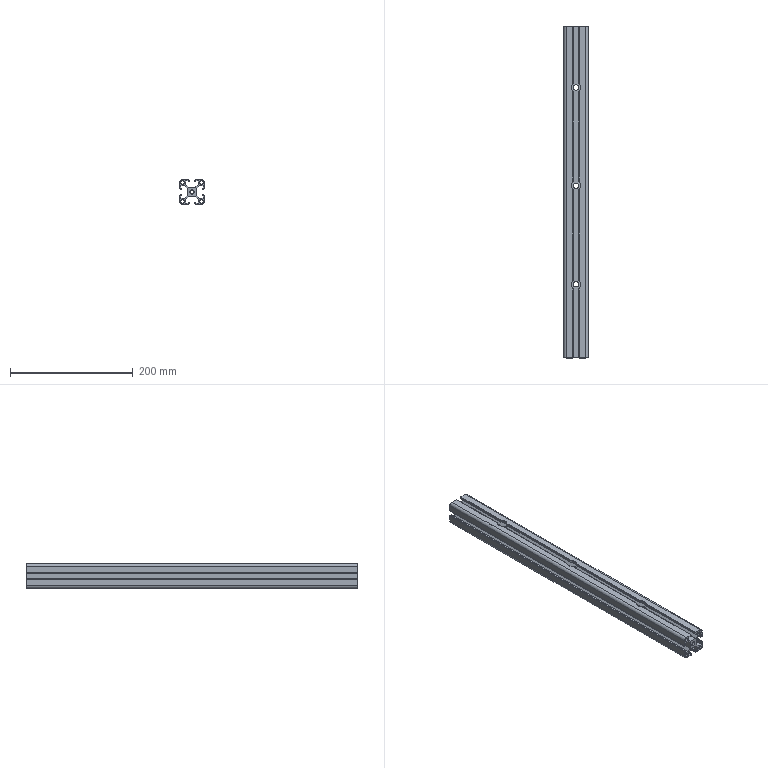Part | SolidWorks | features HoleWzd 1, WeldMemberFeat 1, WeldmentFeature 1 | 1 solid | 167 faces | box 40 x 540 x 40 mm | volume 323932 mm3 | plane 114 | cylinder 53 | commonest cylinder face diameters 9 x19 16 x18 6 x8 6.8 x8